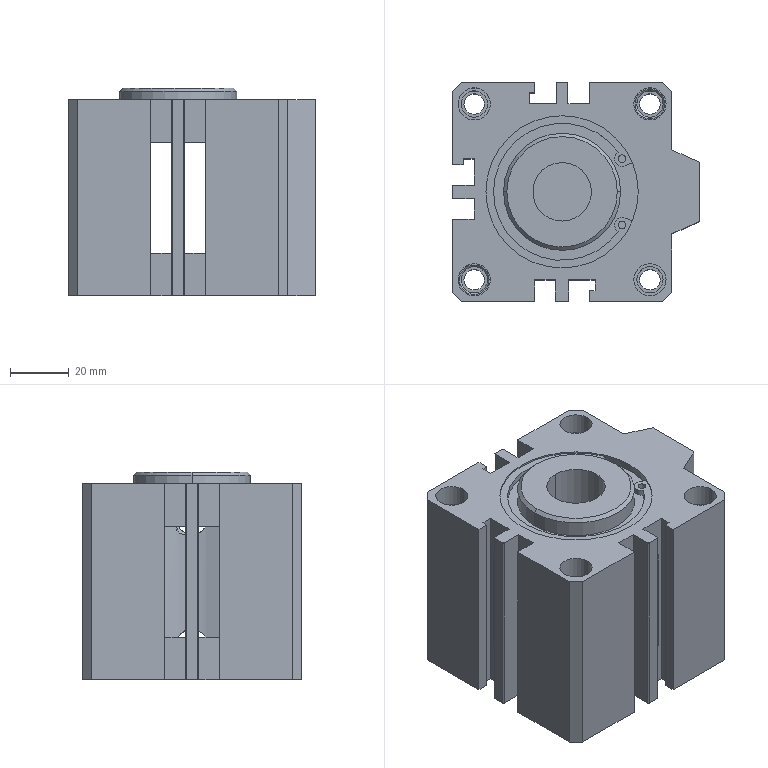Part | SolidWorks | features BaseBody 1 | 1 solid | 193 faces | box 84.5 x 75 x 71 mm | volume 229249 mm3 | cylinder 95 | plane 80 | cone 10 | spline 8 | commonest cylinder face diameters 11 x44 9 x16 0.6 x8 7 x8 2.6 x4 5.2 x4